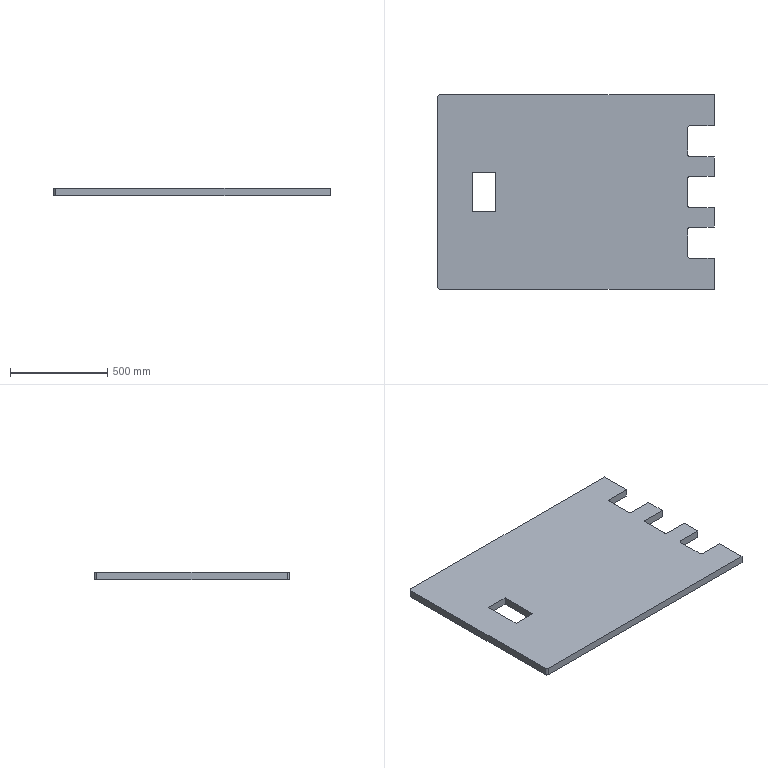Part | SolidWorks | features Extrusion 1, Fillet 1 | 1 solid | 30 faces | box 1420 x 1000 x 40 mm | volume 53251434 mm3 | plane 22 | cylinder 8 | commonest cylinder face diameters 20 x8
STEP:
#1=CARTESIAN_POINT('',(0.,990.,40.));
#2=VERTEX_POINT('',#1);
#3=CARTESIAN_POINT('',(0.,10.,40.));
#4=VERTEX_POINT('',#3);
#5=CARTESIAN_POINT('',(0.,0.,40.));
#6=DIRECTION('',(0.,-1.,0.));
#7=VECTOR('',#6,1000.);
#8=LINE('',#5,#7);
#9=EDGE_CURVE('',#2,#4,#8,.T.);
#10=ORIENTED_EDGE('',*,*,#9,.T.);
#11=CARTESIAN_POINT('',(10.,0.,40.));
#12=VERTEX_POINT('',#11);
#13=CARTESIAN_POINT('',(10.,10.,40.));
#14=DIRECTION('',(0.,0.,1.));
#15=DIRECTION('',(1.,0.,0.));
#16=AXIS2_PLACEMENT_3D('',#13,#14,#15);
#17=CIRCLE('',#16,10.);
#18=EDGE_CURVE('',#4,#12,#17,.T.);
#19=ORIENTED_EDGE('',*,*,#18,.T.);
#20=CARTESIAN_POINT('',(1420.,0.,40.));
#21=VERTEX_POINT('',#20);
#22=CARTESIAN_POINT('',(0.,0.,40.));
#23=DIRECTION('',(1.,0.,0.));
#24=VECTOR('',#23,1000.);
#25=LINE('',#22,#24);
#26=EDGE_CURVE('',#12,#21,#25,.T.);
#27=ORIENTED_EDGE('',*,*,#26,.T.);
#28=CARTESIAN_POINT('',(1420.,160.,40.));
#29=VERTEX_POINT('',#28);
#30=CARTESIAN_POINT('',(1420.,0.,40.));
#31=DIRECTION('',(0.,1.,0.));
#32=VECTOR('',#31,1000.);
#33=LINE('',#30,#32);
#34=EDGE_CURVE('',#21,#29,#33,.T.);
#35=ORIENTED_EDGE('',*,*,#34,.T.);
#36=CARTESIAN_POINT('',(1295.,160.,40.));
#37=VERTEX_POINT('',#36);
#38=CARTESIAN_POINT('',(1295.,160.,40.));
#39=DIRECTION('',(-1.,0.,0.));
#40=VECTOR('',#39,1000.);
#41=LINE('',#38,#40);
#42=EDGE_CURVE('',#29,#37,#41,.T.);
#43=ORIENTED_EDGE('',*,*,#42,.T.);
#44=CARTESIAN_POINT('',(1285.,170.,40.));
#45=VERTEX_POINT('',#44);
#46=CARTESIAN_POINT('',(1295.,170.,40.));
#47=DIRECTION('',(0.,0.,-1.));
#48=DIRECTION('',(1.,0.,0.));
#49=AXIS2_PLACEMENT_3D('',#46,#47,#48);
#50=CIRCLE('',#49,10.);
#51=EDGE_CURVE('',#37,#45,#50,.T.);
#52=ORIENTED_EDGE('',*,*,#51,.T.);
#53=CARTESIAN_POINT('',(1285.,310.,40.));
#54=VERTEX_POINT('',#53);
#55=CARTESIAN_POINT('',(1285.,310.,40.));
#56=DIRECTION('',(0.,1.,0.));
#57=VECTOR('',#56,1000.);
#58=LINE('',#55,#57);
#59=EDGE_CURVE('',#45,#54,#58,.T.);
#60=ORIENTED_EDGE('',*,*,#59,.T.);
#61=CARTESIAN_POINT('',(1295.,320.,40.));
#62=VERTEX_POINT('',#61);
#63=CARTESIAN_POINT('',(1295.,310.,40.));
#64=DIRECTION('',(0.,0.,-1.));
#65=DIRECTION('',(1.,0.,0.));
#66=AXIS2_PLACEMENT_3D('',#63,#64,#65);
#67=CIRCLE('',#66,10.);
#68=EDGE_CURVE('',#54,#62,#67,.T.);
#69=ORIENTED_EDGE('',*,*,#68,.T.);
#70=CARTESIAN_POINT('',(1420.,320.,40.));
#71=VERTEX_POINT('',#70);
#72=CARTESIAN_POINT('',(1420.,320.,40.));
#73=DIRECTION('',(1.,0.,0.));
#74=VECTOR('',#73,1000.);
#75=LINE('',#72,#74);
#76=EDGE_CURVE('',#62,#71,#75,.T.);
#77=ORIENTED_EDGE('',*,*,#76,.T.);
#78=CARTESIAN_POINT('',(1420.,420.,40.));
#79=VERTEX_POINT('',#78);
#80=CARTESIAN_POINT('',(1420.,320.,40.));
#81=DIRECTION('',(0.,1.,0.));
#82=VECTOR('',#81,1000.);
#83=LINE('',#80,#82);
#84=EDGE_CURVE('',#71,#79,#83,.T.);
#85=ORIENTED_EDGE('',*,*,#84,.T.);
#86=CARTESIAN_POINT('',(1295.,420.,40.));
#87=VERTEX_POINT('',#86);
#88=CARTESIAN_POINT('',(1295.,420.,40.));
#89=DIRECTION('',(-1.,0.,0.));
#90=VECTOR('',#89,1000.);
#91=LINE('',#88,#90);
#92=EDGE_CURVE('',#79,#87,#91,.T.);
#93=ORIENTED_EDGE('',*,*,#92,.T.);
#94=CARTESIAN_POINT('',(1285.,430.,40.));
#95=VERTEX_POINT('',#94);
#96=CARTESIAN_POINT('',(1295.,430.,40.));
#97=DIRECTION('',(0.,0.,-1.));
#98=DIRECTION('',(1.,0.,0.));
#99=AXIS2_PLACEMENT_3D('',#96,#97,#98);
#100=CIRCLE('',#99,10.);
#101=EDGE_CURVE('',#87,#95,#100,.T.);
#102=ORIENTED_EDGE('',*,*,#101,.T.);
#103=CARTESIAN_POINT('',(1285.,570.,40.));
#104=VERTEX_POINT('',#103);
#105=CARTESIAN_POINT('',(1285.,570.,40.));
#106=DIRECTION('',(0.,1.,0.));
#107=VECTOR('',#106,1000.);
#108=LINE('',#105,#107);
#109=EDGE_CURVE('',#95,#104,#108,.T.);
#110=ORIENTED_EDGE('',*,*,#109,.T.);
#111=CARTESIAN_POINT('',(1295.,580.,40.));
#112=VERTEX_POINT('',#111);
#113=CARTESIAN_POINT('',(1295.,570.,40.));
#114=DIRECTION('',(0.,0.,-1.));
#115=DIRECTION('',(1.,0.,0.));
#116=AXIS2_PLACEMENT_3D('',#113,#114,#115);
#117=CIRCLE('',#116,10.);
#118=EDGE_CURVE('',#104,#112,#117,.T.);
#119=ORIENTED_EDGE('',*,*,#118,.T.);
#120=CARTESIAN_POINT('',(1420.,580.,40.));
#121=VERTEX_POINT('',#120);
#122=CARTESIAN_POINT('',(1420.,580.,40.));
#123=DIRECTION('',(1.,0.,0.));
#124=VECTOR('',#123,1000.);
#125=LINE('',#122,#124);
#126=EDGE_CURVE('',#112,#121,#125,.T.);
#127=ORIENTED_EDGE('',*,*,#126,.T.);
#128=CARTESIAN_POINT('',(1420.,680.,40.));
#129=VERTEX_POINT('',#128);
#130=CARTESIAN_POINT('',(1420.,580.,40.));
#131=DIRECTION('',(0.,1.,0.));
#132=VECTOR('',#131,1000.);
#133=LINE('',#130,#132);
#134=EDGE_CURVE('',#121,#129,#133,.T.);
#135=ORIENTED_EDGE('',*,*,#134,.T.);
#136=CARTESIAN_POINT('',(1295.,680.,40.));
#137=VERTEX_POINT('',#136);
#138=CARTESIAN_POINT('',(1295.,680.,40.));
#139=DIRECTION('',(-1.,0.,0.));
#140=VECTOR('',#139,1000.);
#141=LINE('',#138,#140);
#142=EDGE_CURVE('',#129,#137,#141,.T.);
#143=ORIENTED_EDGE('',*,*,#142,.T.);
#144=CARTESIAN_POINT('',(1285.,690.,40.));
#145=VERTEX_POINT('',#144);
#146=CARTESIAN_POINT('',(1295.,690.,40.));
#147=DIRECTION('',(0.,0.,-1.));
#148=DIRECTION('',(1.,0.,0.));
#149=AXIS2_PLACEMENT_3D('',#146,#147,#148);
#150=CIRCLE('',#149,10.);
#151=EDGE_CURVE('',#137,#145,#150,.T.);
#152=ORIENTED_EDGE('',*,*,#151,.T.);
#153=CARTESIAN_POINT('',(1285.,830.,40.));
#154=VERTEX_POINT('',#153);
#155=CARTESIAN_POINT('',(1285.,830.,40.));
#156=DIRECTION('',(0.,1.,0.));
#157=VECTOR('',#156,1000.);
#158=LINE('',#155,#157);
#159=EDGE_CURVE('',#145,#154,#158,.T.);
#160=ORIENTED_EDGE('',*,*,#159,.T.);
#161=CARTESIAN_POINT('',(1295.,840.,40.));
#162=VERTEX_POINT('',#161);
#163=CARTESIAN_POINT('',(1295.,830.,40.));
#164=DIRECTION('',(0.,0.,-1.));
#165=DIRECTION('',(1.,0.,0.));
#166=AXIS2_PLACEMENT_3D('',#163,#164,#165);
#167=CIRCLE('',#166,10.);
#168=EDGE_CURVE('',#154,#162,#167,.T.);
#169=ORIENTED_EDGE('',*,*,#168,.T.);
#170=CARTESIAN_POINT('',(1420.,840.,40.));
#171=VERTEX_POINT('',#170);
#172=CARTESIAN_POINT('',(1420.,840.,40.));
#173=DIRECTION('',(1.,0.,0.));
#174=VECTOR('',#173,1000.);
#175=LINE('',#172,#174);
#176=EDGE_CURVE('',#162,#171,#175,.T.);
#177=ORIENTED_EDGE('',*,*,#176,.T.);
#178=CARTESIAN_POINT('',(1420.,1000.,40.));
#179=VERTEX_POINT('',#178);
#180=CARTESIAN_POINT('',(1420.,840.,40.));
#181=DIRECTION('',(0.,1.,0.));
#182=VECTOR('',#181,1000.);
#183=LINE('',#180,#182);
#184=EDGE_CURVE('',#171,#179,#183,.T.);
#185=ORIENTED_EDGE('',*,*,#184,.T.);
#186=CARTESIAN_POINT('',(10.,1000.,40.));
#187=VERTEX_POINT('',#186);
#188=CARTESIAN_POINT('',(0.,1000.,40.));
#189=DIRECTION('',(-1.,0.,0.));
#190=VECTOR('',#189,1000.);
#191=LINE('',#188,#190);
#192=EDGE_CURVE('',#179,#187,#191,.T.);
#193=ORIENTED_EDGE('',*,*,#192,.T.);
#194=CARTESIAN_POINT('',(10.,990.,40.));
#195=DIRECTION('',(0.,0.,1.));
#196=DIRECTION('',(1.,0.,0.));
#197=AXIS2_PLACEMENT_3D('',#194,#195,#196);
#198=CIRCLE('',#197,10.);
#199=EDGE_CURVE('',#187,#2,#198,.T.);
#200=ORIENTED_EDGE('',*,*,#199,.T.);
#201=EDGE_LOOP('',(#10,#19,#27,#35,#43,#52,#60,#69,#77,#85,#93,#102,#110,#119,#127,#135,#143,#152,#160,#169,#177,#185,#193,#200));
#202=FACE_OUTER_BOUND('',#201,.T.);
#203=CARTESIAN_POINT('',(177.,400.,40.));
#204=VERTEX_POINT('',#203);
#205=CARTESIAN_POINT('',(297.,400.,40.));
#206=VERTEX_POINT('',#205);
#207=CARTESIAN_POINT('',(177.,400.,40.));
#208=DIRECTION('',(1.,0.,0.));
#209=VECTOR('',#208,1000.);
#210=LINE('',#207,#209);
#211=EDGE_CURVE('',#204,#206,#210,.T.);
#212=ORIENTED_EDGE('',*,*,#211,.F.);
#213=CARTESIAN_POINT('',(177.,600.,40.));
#214=VERTEX_POINT('',#213);
#215=CARTESIAN_POINT('',(177.,600.,40.));
#216=DIRECTION('',(0.,-1.,0.));
#217=VECTOR('',#216,1000.);
#218=LINE('',#215,#217);
#219=EDGE_CURVE('',#214,#204,#218,.T.);
#220=ORIENTED_EDGE('',*,*,#219,.F.);
#221=CARTESIAN_POINT('',(297.,600.,40.));
#222=VERTEX_POINT('',#221);
#223=CARTESIAN_POINT('',(177.,600.,40.));
#224=DIRECTION('',(-1.,0.,0.));
#225=VECTOR('',#224,1000.);
#226=LINE('',#223,#225);
#227=EDGE_CURVE('',#222,#214,#226,.T.);
#228=ORIENTED_EDGE('',*,*,#227,.F.);
#229=CARTESIAN_POINT('',(297.,600.,40.));
#230=DIRECTION('',(0.,1.,0.));
#231=VECTOR('',#230,1000.);
#232=LINE('',#229,#231);
#233=EDGE_CURVE('',#206,#222,#232,.T.);
#234=ORIENTED_EDGE('',*,*,#233,.F.);
#235=EDGE_LOOP('',(#212,#220,#228,#234));
#236=FACE_BOUND('',#235,.T.);
#237=CARTESIAN_POINT('',(1295.,830.,40.));
#238=DIRECTION('',(0.,0.,1.));
#239=DIRECTION('',(1.,0.,0.));
#240=AXIS2_PLACEMENT_3D('',#237,#238,#239);
#241=PLANE('',#240);
#242=ADVANCED_FACE('',(#202,#236),#241,.T.);
#243=CARTESIAN_POINT('',(10.,0.,0.));
#244=VERTEX_POINT('',#243);
#245=CARTESIAN_POINT('',(1420.,0.,0.));
#246=VERTEX_POINT('',#245);
#247=CARTESIAN_POINT('',(0.,0.,0.));
#248=DIRECTION('',(1.,0.,0.));
#249=VECTOR('',#248,1000.);
#250=LINE('',#247,#249);
#251=EDGE_CURVE('',#244,#246,#250,.T.);
#252=ORIENTED_EDGE('',*,*,#251,.F.);
#253=CARTESIAN_POINT('',(0.,10.,0.));
#254=VERTEX_POINT('',#253);
#255=CARTESIAN_POINT('',(10.,10.,0.));
#256=DIRECTION('',(0.,0.,-1.));
#257=DIRECTION('',(1.,0.,0.));
#258=AXIS2_PLACEMENT_3D('',#255,#256,#257);
#259=CIRCLE('',#258,10.);
#260=EDGE_CURVE('',#244,#254,#259,.T.);
#261=ORIENTED_EDGE('',*,*,#260,.T.);
#262=CARTESIAN_POINT('',(0.,990.,0.));
#263=VERTEX_POINT('',#262);
#264=CARTESIAN_POINT('',(0.,0.,0.));
#265=DIRECTION('',(0.,-1.,0.));
#266=VECTOR('',#265,1000.);
#267=LINE('',#264,#266);
#268=EDGE_CURVE('',#263,#254,#267,.T.);
#269=ORIENTED_EDGE('',*,*,#268,.F.);
#270=CARTESIAN_POINT('',(10.,1000.,0.));
#271=VERTEX_POINT('',#270);
#272=CARTESIAN_POINT('',(10.,990.,0.));
#273=DIRECTION('',(0.,0.,-1.));
#274=DIRECTION('',(1.,0.,0.));
#275=AXIS2_PLACEMENT_3D('',#272,#273,#274);
#276=CIRCLE('',#275,10.);
#277=EDGE_CURVE('',#263,#271,#276,.T.);
#278=ORIENTED_EDGE('',*,*,#277,.T.);
#279=CARTESIAN_POINT('',(1420.,1000.,0.));
#280=VERTEX_POINT('',#279);
#281=CARTESIAN_POINT('',(0.,1000.,0.));
#282=DIRECTION('',(-1.,0.,0.));
#283=VECTOR('',#282,1000.);
#284=LINE('',#281,#283);
#285=EDGE_CURVE('',#280,#271,#284,.T.);
#286=ORIENTED_EDGE('',*,*,#285,.F.);
#287=CARTESIAN_POINT('',(1420.,840.,0.));
#288=VERTEX_POINT('',#287);
#289=CARTESIAN_POINT('',(1420.,840.,0.));
#290=DIRECTION('',(0.,1.,0.));
#291=VECTOR('',#290,1000.);
#292=LINE('',#289,#291);
#293=EDGE_CURVE('',#288,#280,#292,.T.);
#294=ORIENTED_EDGE('',*,*,#293,.F.);
#295=CARTESIAN_POINT('',(1295.,840.,0.));
#296=VERTEX_POINT('',#295);
#297=CARTESIAN_POINT('',(1420.,840.,0.));
#298=DIRECTION('',(1.,0.,0.));
#299=VECTOR('',#298,1000.);
#300=LINE('',#297,#299);
#301=EDGE_CURVE('',#296,#288,#300,.T.);
#302=ORIENTED_EDGE('',*,*,#301,.F.);
#303=CARTESIAN_POINT('',(1285.,830.,0.));
#304=VERTEX_POINT('',#303);
#305=CARTESIAN_POINT('',(1295.,830.,0.));
#306=DIRECTION('',(0.,0.,-1.));
#307=DIRECTION('',(1.,0.,0.));
#308=AXIS2_PLACEMENT_3D('',#305,#306,#307);
#309=CIRCLE('',#308,10.);
#310=EDGE_CURVE('',#304,#296,#309,.T.);
#311=ORIENTED_EDGE('',*,*,#310,.F.);
#312=CARTESIAN_POINT('',(1285.,690.,0.));
#313=VERTEX_POINT('',#312);
#314=CARTESIAN_POINT('',(1285.,830.,0.));
#315=DIRECTION('',(0.,1.,0.));
#316=VECTOR('',#315,1000.);
#317=LINE('',#314,#316);
#318=EDGE_CURVE('',#313,#304,#317,.T.);
#319=ORIENTED_EDGE('',*,*,#318,.F.);
#320=CARTESIAN_POINT('',(1295.,680.,0.));
#321=VERTEX_POINT('',#320);
#322=CARTESIAN_POINT('',(1295.,690.,0.));
#323=DIRECTION('',(0.,0.,-1.));
#324=DIRECTION('',(1.,0.,0.));
#325=AXIS2_PLACEMENT_3D('',#322,#323,#324);
#326=CIRCLE('',#325,10.);
#327=EDGE_CURVE('',#321,#313,#326,.T.);
#328=ORIENTED_EDGE('',*,*,#327,.F.);
#329=CARTESIAN_POINT('',(1420.,680.,0.));
#330=VERTEX_POINT('',#329);
#331=CARTESIAN_POINT('',(1295.,680.,0.));
#332=DIRECTION('',(-1.,0.,0.));
#333=VECTOR('',#332,1000.);
#334=LINE('',#331,#333);
#335=EDGE_CURVE('',#330,#321,#334,.T.);
#336=ORIENTED_EDGE('',*,*,#335,.F.);
#337=CARTESIAN_POINT('',(1420.,580.,0.));
#338=VERTEX_POINT('',#337);
#339=CARTESIAN_POINT('',(1420.,580.,0.));
#340=DIRECTION('',(0.,1.,0.));
#341=VECTOR('',#340,1000.);
#342=LINE('',#339,#341);
#343=EDGE_CURVE('',#338,#330,#342,.T.);
#344=ORIENTED_EDGE('',*,*,#343,.F.);
#345=CARTESIAN_POINT('',(1295.,580.,0.));
#346=VERTEX_POINT('',#345);
#347=CARTESIAN_POINT('',(1420.,580.,0.));
#348=DIRECTION('',(1.,0.,0.));
#349=VECTOR('',#348,1000.);
#350=LINE('',#347,#349);
#351=EDGE_CURVE('',#346,#338,#350,.T.);
#352=ORIENTED_EDGE('',*,*,#351,.F.);
#353=CARTESIAN_POINT('',(1285.,570.,0.));
#354=VERTEX_POINT('',#353);
#355=CARTESIAN_POINT('',(1295.,570.,0.));
#356=DIRECTION('',(0.,0.,-1.));
#357=DIRECTION('',(1.,0.,0.));
#358=AXIS2_PLACEMENT_3D('',#355,#356,#357);
#359=CIRCLE('',#358,10.);
#360=EDGE_CURVE('',#354,#346,#359,.T.);
#361=ORIENTED_EDGE('',*,*,#360,.F.);
#362=CARTESIAN_POINT('',(1285.,430.,0.));
#363=VERTEX_POINT('',#362);
#364=CARTESIAN_POINT('',(1285.,570.,0.));
#365=DIRECTION('',(0.,1.,0.));
#366=VECTOR('',#365,1000.);
#367=LINE('',#364,#366);
#368=EDGE_CURVE('',#363,#354,#367,.T.);
#369=ORIENTED_EDGE('',*,*,#368,.F.);
#370=CARTESIAN_POINT('',(1295.,420.,0.));
#371=VERTEX_POINT('',#370);
#372=CARTESIAN_POINT('',(1295.,430.,0.));
#373=DIRECTION('',(0.,0.,-1.));
#374=DIRECTION('',(1.,0.,0.));
#375=AXIS2_PLACEMENT_3D('',#372,#373,#374);
#376=CIRCLE('',#375,10.);
#377=EDGE_CURVE('',#371,#363,#376,.T.);
#378=ORIENTED_EDGE('',*,*,#377,.F.);
#379=CARTESIAN_POINT('',(1420.,420.,0.));
#380=VERTEX_POINT('',#379);
#381=CARTESIAN_POINT('',(1295.,420.,0.));
#382=DIRECTION('',(-1.,0.,0.));
#383=VECTOR('',#382,1000.);
#384=LINE('',#381,#383);
#385=EDGE_CURVE('',#380,#371,#384,.T.);
#386=ORIENTED_EDGE('',*,*,#385,.F.);
#387=CARTESIAN_POINT('',(1420.,320.,0.));
#388=VERTEX_POINT('',#387);
#389=CARTESIAN_POINT('',(1420.,320.,0.));
#390=DIRECTION('',(0.,1.,0.));
#391=VECTOR('',#390,1000.);
#392=LINE('',#389,#391);
#393=EDGE_CURVE('',#388,#380,#392,.T.);
#394=ORIENTED_EDGE('',*,*,#393,.F.);
#395=CARTESIAN_POINT('',(1295.,320.,0.));
#396=VERTEX_POINT('',#395);
#397=CARTESIAN_POINT('',(1420.,320.,0.));
#398=DIRECTION('',(1.,0.,0.));
#399=VECTOR('',#398,1000.);
#400=LINE('',#397,#399);
#401=EDGE_CURVE('',#396,#388,#400,.T.);
#402=ORIENTED_EDGE('',*,*,#401,.F.);
#403=CARTESIAN_POINT('',(1285.,310.,0.));
#404=VERTEX_POINT('',#403);
#405=CARTESIAN_POINT('',(1295.,310.,0.));
#406=DIRECTION('',(0.,0.,-1.));
#407=DIRECTION('',(1.,0.,0.));
#408=AXIS2_PLACEMENT_3D('',#405,#406,#407);
#409=CIRCLE('',#408,10.);
#410=EDGE_CURVE('',#404,#396,#409,.T.);
#411=ORIENTED_EDGE('',*,*,#410,.F.);
#412=CARTESIAN_POINT('',(1285.,170.,0.));
#413=VERTEX_POINT('',#412);
#414=CARTESIAN_POINT('',(1285.,310.,0.));
#415=DIRECTION('',(0.,1.,0.));
#416=VECTOR('',#415,1000.);
#417=LINE('',#414,#416);
#418=EDGE_CURVE('',#413,#404,#417,.T.);
#419=ORIENTED_EDGE('',*,*,#418,.F.);
#420=CARTESIAN_POINT('',(1295.,160.,0.));
#421=VERTEX_POINT('',#420);
#422=CARTESIAN_POINT('',(1295.,170.,0.));
#423=DIRECTION('',(0.,0.,-1.));
#424=DIRECTION('',(1.,0.,0.));
#425=AXIS2_PLACEMENT_3D('',#422,#423,#424);
#426=CIRCLE('',#425,10.);
#427=EDGE_CURVE('',#421,#413,#426,.T.);
#428=ORIENTED_EDGE('',*,*,#427,.F.);
#429=CARTESIAN_POINT('',(1420.,160.,0.));
#430=VERTEX_POINT('',#429);
#431=CARTESIAN_POINT('',(1295.,160.,0.));
#432=DIRECTION('',(-1.,0.,0.));
#433=VECTOR('',#432,1000.);
#434=LINE('',#431,#433);
#435=EDGE_CURVE('',#430,#421,#434,.T.);
#436=ORIENTED_EDGE('',*,*,#435,.F.);
#437=CARTESIAN_POINT('',(1420.,0.,0.));
#438=DIRECTION('',(0.,1.,0.));
#439=VECTOR('',#438,1000.);
#440=LINE('',#437,#439);
#441=EDGE_CURVE('',#246,#430,#440,.T.);
#442=ORIENTED_EDGE('',*,*,#441,.F.);
#443=EDGE_LOOP('',(#252,#261,#269,#278,#286,#294,#302,#311,#319,#328,#336,#344,#352,#361,#369,#378,#386,#394,#402,#411,#419,#428,#436,#442));
#444=FACE_OUTER_BOUND('',#443,.T.);
#445=CARTESIAN_POINT('',(177.,600.,0.));
#446=VERTEX_POINT('',#445);
#447=CARTESIAN_POINT('',(177.,400.,0.));
#448=VERTEX_POINT('',#447);
#449=CARTESIAN_POINT('',(177.,600.,0.));
#450=DIRECTION('',(0.,-1.,0.));
#451=VECTOR('',#450,1000.);
#452=LINE('',#449,#451);
#453=EDGE_CURVE('',#446,#448,#452,.T.);
#454=ORIENTED_EDGE('',*,*,#453,.T.);
#455=CARTESIAN_POINT('',(297.,400.,0.));
#456=VERTEX_POINT('',#455);
#457=CARTESIAN_POINT('',(177.,400.,0.));
#458=DIRECTION('',(1.,0.,0.));
#459=VECTOR('',#458,1000.);
#460=LINE('',#457,#459);
#461=EDGE_CURVE('',#448,#456,#460,.T.);
#462=ORIENTED_EDGE('',*,*,#461,.T.);
#463=CARTESIAN_POINT('',(297.,600.,0.));
#464=VERTEX_POINT('',#463);
#465=CARTESIAN_POINT('',(297.,600.,0.));
#466=DIRECTION('',(0.,1.,0.));
#467=VECTOR('',#466,1000.);
#468=LINE('',#465,#467);
#469=EDGE_CURVE('',#456,#464,#468,.T.);
#470=ORIENTED_EDGE('',*,*,#469,.T.);
#471=CARTESIAN_POINT('',(177.,600.,0.));
#472=DIRECTION('',(-1.,0.,0.));
#473=VECTOR('',#472,1000.);
#474=LINE('',#471,#473);
#475=EDGE_CURVE('',#464,#446,#474,.T.);
#476=ORIENTED_EDGE('',*,*,#475,.T.);
#477=EDGE_LOOP('',(#454,#462,#470,#476));
#478=FACE_BOUND('',#477,.T.);
#479=CARTESIAN_POINT('',(1295.,830.,0.));
#480=DIRECTION('',(0.,0.,1.));
#481=DIRECTION('',(1.,0.,0.));
#482=AXIS2_PLACEMENT_3D('',#479,#480,#481);
#483=PLANE('',#482);
#484=ADVANCED_FACE('',(#444,#478),#483,.F.);
#485=ORIENTED_EDGE('',*,*,#268,.T.);
#486=CARTESIAN_POINT('',(0.,10.,40.));
#487=DIRECTION('',(0.,0.,1.));
#488=VECTOR('',#487,1000.);
#489=LINE('',#486,#488);
#490=EDGE_CURVE('',#254,#4,#489,.T.);
#491=ORIENTED_EDGE('',*,*,#490,.T.);
#492=ORIENTED_EDGE('',*,*,#9,.F.);
#493=CARTESIAN_POINT('',(0.,990.,40.));
#494=DIRECTION('',(0.,0.,-1.));
#495=VECTOR('',#494,1000.);
#496=LINE('',#493,#495);
#497=EDGE_CURVE('',#2,#263,#496,.T.);
#498=ORIENTED_EDGE('',*,*,#497,.T.);
#499=EDGE_LOOP('',(#485,#491,#492,#498));
#500=FACE_OUTER_BOUND('',#499,.T.);
#501=CARTESIAN_POINT('',(0.,0.,40.));
#502=DIRECTION('',(1.,0.,0.));
#503=DIRECTION('',(0.,0.,-1.));
#504=AXIS2_PLACEMENT_3D('',#501,#502,#503);
#505=PLANE('',#504);
#506=ADVANCED_FACE('',(#500),#505,.F.);
#507=ORIENTED_EDGE('',*,*,#26,.F.);
#508=CARTESIAN_POINT('',(10.,0.,40.));
#509=DIRECTION('',(0.,0.,-1.));
#510=VECTOR('',#509,1000.);
#511=LINE('',#508,#510);
#512=EDGE_CURVE('',#12,#244,#511,.T.);
#513=ORIENTED_EDGE('',*,*,#512,.T.);
#514=ORIENTED_EDGE('',*,*,#251,.T.);
#515=CARTESIAN_POINT('',(1420.,0.,40.));
#516=DIRECTION('',(0.,0.,-1.));
#517=VECTOR('',#516,1000.);
#518=LINE('',#515,#517);
#519=EDGE_CURVE('',#21,#246,#518,.T.);
#520=ORIENTED_EDGE('',*,*,#519,.F.);
#521=EDGE_LOOP('',(#507,#513,#514,#520));
#522=FACE_OUTER_BOUND('',#521,.T.);
#523=CARTESIAN_POINT('',(0.,0.,40.));
#524=DIRECTION('',(0.,1.,0.));
#525=DIRECTION('',(0.,0.,1.));
#526=AXIS2_PLACEMENT_3D('',#523,#524,#525);
#527=PLANE('',#526);
#528=ADVANCED_FACE('',(#522),#527,.F.);
#529=ORIENTED_EDGE('',*,*,#441,.T.);
#530=CARTESIAN_POINT('',(1420.,160.,40.));
#531=DIRECTION('',(0.,0.,-1.));
#532=VECTOR('',#531,1000.);
#533=LINE('',#530,#532);
#534=EDGE_CURVE('',#29,#430,#533,.T.);
#535=ORIENTED_EDGE('',*,*,#534,.F.);
#536=ORIENTED_EDGE('',*,*,#34,.F.);
#537=ORIENTED_EDGE('',*,*,#519,.T.);
#538=EDGE_LOOP('',(#529,#535,#536,#537));
#539=FACE_OUTER_BOUND('',#538,.T.);
#540=CARTESIAN_POINT('',(1420.,0.,40.));
#541=DIRECTION('',(-1.,0.,0.));
#542=DIRECTION('',(0.,0.,1.));
#543=AXIS2_PLACEMENT_3D('',#540,#541,#542);
#544=PLANE('',#543);
#545=ADVANCED_FACE('',(#539),#544,.F.);
#546=ORIENTED_EDGE('',*,*,#435,.T.);
#547=CARTESIAN_POINT('',(1295.,160.,40.));
#548=DIRECTION('',(0.,0.,-1.));
#549=VECTOR('',#548,1000.);
#550=LINE('',#547,#549);
#551=EDGE_CURVE('',#37,#421,#550,.T.);
#552=ORIENTED_EDGE('',*,*,#551,.F.);
#553=ORIENTED_EDGE('',*,*,#42,.F.);
#554=ORIENTED_EDGE('',*,*,#534,.T.);
#555=EDGE_LOOP('',(#546,#552,#553,#554));
#556=FACE_OUTER_BOUND('',#555,.T.);
#557=CARTESIAN_POINT('',(1295.,160.,40.));
#558=DIRECTION('',(0.,-1.,0.));
#559=DIRECTION('',(0.,0.,-1.));
#560=AXIS2_PLACEMENT_3D('',#557,#558,#559);
#561=PLANE('',#560);
#562=ADVANCED_FACE('',(#556),#561,.F.);
#563=ORIENTED_EDGE('',*,*,#427,.T.);
#564=CARTESIAN_POINT('',(1285.,170.,40.));
#565=DIRECTION('',(0.,0.,-1.));
#566=VECTOR('',#565,1000.);
#567=LINE('',#564,#566);
#568=EDGE_CURVE('',#45,#413,#567,.T.);
#569=ORIENTED_EDGE('',*,*,#568,.F.);
#570=ORIENTED_EDGE('',*,*,#51,.F.);
#571=ORIENTED_EDGE('',*,*,#551,.T.);
#572=EDGE_LOOP('',(#563,#569,#570,#571));
#573=FACE_OUTER_BOUND('',#572,.T.);
#574=CARTESIAN_POINT('',(1295.,170.,40.));
#575=DIRECTION('',(0.,0.,-1.));
#576=DIRECTION('',(-1.,0.,0.));
#577=AXIS2_PLACEMENT_3D('',#574,#575,#576);
#578=CYLINDRICAL_SURFACE('',#577,10.);
#579=ADVANCED_FACE('',(#573),#578,.F.);
#580=ORIENTED_EDGE('',*,*,#418,.T.);
#581=CARTESIAN_POINT('',(1285.,310.,40.));
#582=DIRECTION('',(0.,0.,-1.));
#583=VECTOR('',#582,1000.);
#584=LINE('',#581,#583);
#585=EDGE_CURVE('',#54,#404,#584,.T.);
#586=ORIENTED_EDGE('',*,*,#585,.F.);
#587=ORIENTED_EDGE('',*,*,#59,.F.);
#588=ORIENTED_EDGE('',*,*,#568,.T.);
#589=EDGE_LOOP('',(#580,#586,#587,#588));
#590=FACE_OUTER_BOUND('',#589,.T.);
#591=CARTESIAN_POINT('',(1285.,310.,40.));
#592=DIRECTION('',(-1.,0.,0.));
#593=DIRECTION('',(0.,0.,1.));
#594=AXIS2_PLACEMENT_3D('',#591,#592,#593);
#595=PLANE('',#594);
#596=ADVANCED_FACE('',(#590),#595,.F.);
#597=ORIENTED_EDGE('',*,*,#410,.T.);
#598=CARTESIAN_POINT('',(1295.,320.,40.));
#599=DIRECTION('',(0.,0.,-1.));
#600=VECTOR('',#599,1000.);
#601=LINE('',#598,#600);
#602=EDGE_CURVE('',#62,#396,#601,.T.);
#603=ORIENTED_EDGE('',*,*,#602,.F.);
#604=ORIENTED_EDGE('',*,*,#68,.F.);
#605=ORIENTED_EDGE('',*,*,#585,.T.);
#606=EDGE_LOOP('',(#597,#603,#604,#605));
#607=FACE_OUTER_BOUND('',#606,.T.);
#608=CARTESIAN_POINT('',(1295.,310.,40.));
#609=DIRECTION('',(0.,0.,-1.));
#610=DIRECTION('',(-1.,0.,0.));
#611=AXIS2_PLACEMENT_3D('',#608,#609,#610);
#612=CYLINDRICAL_SURFACE('',#611,10.);
#613=ADVANCED_FACE('',(#607),#612,.F.);
#614=ORIENTED_EDGE('',*,*,#401,.T.);
#615=CARTESIAN_POINT('',(1420.,320.,40.));
#616=DIRECTION('',(0.,0.,-1.));
#617=VECTOR('',#616,1000.);
#618=LINE('',#615,#617);
#619=EDGE_CURVE('',#71,#388,#618,.T.);
#620=ORIENTED_EDGE('',*,*,#619,.F.);
#621=ORIENTED_EDGE('',*,*,#76,.F.);
#622=ORIENTED_EDGE('',*,*,#602,.T.);
#623=EDGE_LOOP('',(#614,#620,#621,#622));
#624=FACE_OUTER_BOUND('',#623,.T.);
#625=CARTESIAN_POINT('',(1420.,320.,40.));
#626=DIRECTION('',(0.,1.,0.));
#627=DIRECTION('',(-1.,0.,0.));
#628=AXIS2_PLACEMENT_3D('',#625,#626,#627);
#629=PLANE('',#628);
#630=ADVANCED_FACE('',(#624),#629,.F.);
#631=ORIENTED_EDGE('',*,*,#393,.T.);
#632=CARTESIAN_POINT('',(1420.,420.,40.));
#633=DIRECTION('',(0.,0.,-1.));
#634=VECTOR('',#633,1000.);
#635=LINE('',#632,#634);
#636=EDGE_CURVE('',#79,#380,#635,.T.);
#637=ORIENTED_EDGE('',*,*,#636,.F.);
#638=ORIENTED_EDGE('',*,*,#84,.F.);
#639=ORIENTED_EDGE('',*,*,#619,.T.);
#640=EDGE_LOOP('',(#631,#637,#638,#639));
#641=FACE_OUTER_BOUND('',#640,.T.);
#642=CARTESIAN_POINT('',(1420.,320.,40.));
#643=DIRECTION('',(-1.,0.,0.));
#644=DIRECTION('',(0.,-1.,0.));
#645=AXIS2_PLACEMENT_3D('',#642,#643,#644);
#646=PLANE('',#645);
#647=ADVANCED_FACE('',(#641),#646,.F.);
#648=ORIENTED_EDGE('',*,*,#385,.T.);
#649=CARTESIAN_POINT('',(1295.,420.,40.));
#650=DIRECTION('',(0.,0.,-1.));
#651=VECTOR('',#650,1000.);
#652=LINE('',#649,#651);
#653=EDGE_CURVE('',#87,#371,#652,.T.);
#654=ORIENTED_EDGE('',*,*,#653,.F.);
#655=ORIENTED_EDGE('',*,*,#92,.F.);
#656=ORIENTED_EDGE('',*,*,#636,.T.);
#657=EDGE_LOOP('',(#648,#654,#655,#656));
#658=FACE_OUTER_BOUND('',#657,.T.);
#659=CARTESIAN_POINT('',(1295.,420.,40.));
#660=DIRECTION('',(0.,-1.,0.));
#661=DIRECTION('',(0.,0.,-1.));
#662=AXIS2_PLACEMENT_3D('',#659,#660,#661);
#663=PLANE('',#662);
#664=ADVANCED_FACE('',(#658),#663,.F.);
#665=ORIENTED_EDGE('',*,*,#377,.T.);
#666=CARTESIAN_POINT('',(1285.,430.,40.));
#667=DIRECTION('',(0.,0.,-1.));
#668=VECTOR('',#667,1000.);
#669=LINE('',#666,#668);
#670=EDGE_CURVE('',#95,#363,#669,.T.);
#671=ORIENTED_EDGE('',*,*,#670,.F.);
#672=ORIENTED_EDGE('',*,*,#101,.F.);
#673=ORIENTED_EDGE('',*,*,#653,.T.);
#674=EDGE_LOOP('',(#665,#671,#672,#673));
#675=FACE_OUTER_BOUND('',#674,.T.);
#676=CARTESIAN_POINT('',(1295.,430.,40.));
#677=DIRECTION('',(0.,0.,-1.));
#678=DIRECTION('',(-1.,0.,0.));
#679=AXIS2_PLACEMENT_3D('',#676,#677,#678);
#680=CYLINDRICAL_SURFACE('',#679,10.);
#681=ADVANCED_FACE('',(#675),#680,.F.);
#682=ORIENTED_EDGE('',*,*,#368,.T.);
#683=CARTESIAN_POINT('',(1285.,570.,40.));
#684=DIRECTION('',(0.,0.,-1.));
#685=VECTOR('',#684,1000.);
#686=LINE('',#683,#685);
#687=EDGE_CURVE('',#104,#354,#686,.T.);
#688=ORIENTED_EDGE('',*,*,#687,.F.);
#689=ORIENTED_EDGE('',*,*,#109,.F.);
#690=ORIENTED_EDGE('',*,*,#670,.T.);
#691=EDGE_LOOP('',(#682,#688,#689,#690));
#692=FACE_OUTER_BOUND('',#691,.T.);
#693=CARTESIAN_POINT('',(1285.,570.,40.));
#694=DIRECTION('',(-1.,0.,0.));
#695=DIRECTION('',(0.,0.,1.));
#696=AXIS2_PLACEMENT_3D('',#693,#694,#695);
#697=PLANE('',#696);
#698=ADVANCED_FACE('',(#692),#697,.F.);
#699=ORIENTED_EDGE('',*,*,#360,.T.);
#700=CARTESIAN_POINT('',(1295.,580.,40.));
#701=DIRECTION('',(0.,0.,-1.));
#702=VECTOR('',#701,1000.);
#703=LINE('',#700,#702);
#704=EDGE_CURVE('',#112,#346,#703,.T.);
#705=ORIENTED_EDGE('',*,*,#704,.F.);
#706=ORIENTED_EDGE('',*,*,#118,.F.);
#707=ORIENTED_EDGE('',*,*,#687,.T.);
#708=EDGE_LOOP('',(#699,#705,#706,#707));
#709=FACE_OUTER_BOUND('',#708,.T.);
#710=CARTESIAN_POINT('',(1295.,570.,40.));
#711=DIRECTION('',(0.,0.,-1.));
#712=DIRECTION('',(-1.,0.,0.));
#713=AXIS2_PLACEMENT_3D('',#710,#711,#712);
#714=CYLINDRICAL_SURFACE('',#713,10.);
#715=ADVANCED_FACE('',(#709),#714,.F.);
#716=ORIENTED_EDGE('',*,*,#351,.T.);
#717=CARTESIAN_POINT('',(1420.,580.,40.));
#718=DIRECTION('',(0.,0.,-1.));
#719=VECTOR('',#718,1000.);
#720=LINE('',#717,#719);
#721=EDGE_CURVE('',#121,#338,#720,.T.);
#722=ORIENTED_EDGE('',*,*,#721,.F.);
#723=ORIENTED_EDGE('',*,*,#126,.F.);
#724=ORIENTED_EDGE('',*,*,#704,.T.);
#725=EDGE_LOOP('',(#716,#722,#723,#724));
#726=FACE_OUTER_BOUND('',#725,.T.);
#727=CARTESIAN_POINT('',(1420.,580.,40.));
#728=DIRECTION('',(0.,1.,0.));
#729=DIRECTION('',(-1.,0.,0.));
#730=AXIS2_PLACEMENT_3D('',#727,#728,#729);
#731=PLANE('',#730);
#732=ADVANCED_FACE('',(#726),#731,.F.);
#733=ORIENTED_EDGE('',*,*,#343,.T.);
#734=CARTESIAN_POINT('',(1420.,680.,40.));
#735=DIRECTION('',(0.,0.,-1.));
#736=VECTOR('',#735,1000.);
#737=LINE('',#734,#736);
#738=EDGE_CURVE('',#129,#330,#737,.T.);
#739=ORIENTED_EDGE('',*,*,#738,.F.);
#740=ORIENTED_EDGE('',*,*,#134,.F.);
#741=ORIENTED_EDGE('',*,*,#721,.T.);
#742=EDGE_LOOP('',(#733,#739,#740,#741));
#743=FACE_OUTER_BOUND('',#742,.T.);
#744=CARTESIAN_POINT('',(1420.,580.,40.));
#745=DIRECTION('',(-1.,0.,0.));
#746=DIRECTION('',(0.,0.,1.));
#747=AXIS2_PLACEMENT_3D('',#744,#745,#746);
#748=PLANE('',#747);
#749=ADVANCED_FACE('',(#743),#748,.F.);
#750=ORIENTED_EDGE('',*,*,#335,.T.);
#751=CARTESIAN_POINT('',(1295.,680.,40.));
#752=DIRECTION('',(0.,0.,-1.));
#753=VECTOR('',#752,1000.);
#754=LINE('',#751,#753);
#755=EDGE_CURVE('',#137,#321,#754,.T.);
#756=ORIENTED_EDGE('',*,*,#755,.F.);
#757=ORIENTED_EDGE('',*,*,#142,.F.);
#758=ORIENTED_EDGE('',*,*,#738,.T.);
#759=EDGE_LOOP('',(#750,#756,#757,#758));
#760=FACE_OUTER_BOUND('',#759,.T.);
#761=CARTESIAN_POINT('',(1295.,680.,40.));
#762=DIRECTION('',(0.,-1.,0.));
#763=DIRECTION('',(0.,0.,-1.));
#764=AXIS2_PLACEMENT_3D('',#761,#762,#763);
#765=PLANE('',#764);
#766=ADVANCED_FACE('',(#760),#765,.F.);
#767=ORIENTED_EDGE('',*,*,#327,.T.);
#768=CARTESIAN_POINT('',(1285.,690.,40.));
#769=DIRECTION('',(0.,0.,-1.));
#770=VECTOR('',#769,1000.);
#771=LINE('',#768,#770);
#772=EDGE_CURVE('',#145,#313,#771,.T.);
#773=ORIENTED_EDGE('',*,*,#772,.F.);
#774=ORIENTED_EDGE('',*,*,#151,.F.);
#775=ORIENTED_EDGE('',*,*,#755,.T.);
#776=EDGE_LOOP('',(#767,#773,#774,#775));
#777=FACE_OUTER_BOUND('',#776,.T.);
#778=CARTESIAN_POINT('',(1295.,690.,40.));
#779=DIRECTION('',(0.,0.,-1.));
#780=DIRECTION('',(-1.,0.,0.));
#781=AXIS2_PLACEMENT_3D('',#778,#779,#780);
#782=CYLINDRICAL_SURFACE('',#781,10.);
#783=ADVANCED_FACE('',(#777),#782,.F.);
#784=ORIENTED_EDGE('',*,*,#318,.T.);
#785=CARTESIAN_POINT('',(1285.,830.,40.));
#786=DIRECTION('',(0.,0.,-1.));
#787=VECTOR('',#786,1000.);
#788=LINE('',#785,#787);
#789=EDGE_CURVE('',#154,#304,#788,.T.);
#790=ORIENTED_EDGE('',*,*,#789,.F.);
#791=ORIENTED_EDGE('',*,*,#159,.F.);
#792=ORIENTED_EDGE('',*,*,#772,.T.);
#793=EDGE_LOOP('',(#784,#790,#791,#792));
#794=FACE_OUTER_BOUND('',#793,.T.);
#795=CARTESIAN_POINT('',(1285.,830.,40.));
#796=DIRECTION('',(-1.,0.,0.));
#797=DIRECTION('',(0.,0.,1.));
#798=AXIS2_PLACEMENT_3D('',#795,#796,#797);
#799=PLANE('',#798);
#800=ADVANCED_FACE('',(#794),#799,.F.);
#801=ORIENTED_EDGE('',*,*,#310,.T.);
#802=CARTESIAN_POINT('',(1295.,840.,40.));
#803=DIRECTION('',(0.,0.,-1.));
#804=VECTOR('',#803,1000.);
#805=LINE('',#802,#804);
#806=EDGE_CURVE('',#162,#296,#805,.T.);
#807=ORIENTED_EDGE('',*,*,#806,.F.);
#808=ORIENTED_EDGE('',*,*,#168,.F.);
#809=ORIENTED_EDGE('',*,*,#789,.T.);
#810=EDGE_LOOP('',(#801,#807,#808,#809));
#811=FACE_OUTER_BOUND('',#810,.T.);
#812=CARTESIAN_POINT('',(1295.,830.,40.));
#813=DIRECTION('',(0.,0.,-1.));
#814=DIRECTION('',(-1.,0.,0.));
#815=AXIS2_PLACEMENT_3D('',#812,#813,#814);
#816=CYLINDRICAL_SURFACE('',#815,10.);
#817=ADVANCED_FACE('',(#811),#816,.F.);
#818=ORIENTED_EDGE('',*,*,#301,.T.);
#819=CARTESIAN_POINT('',(1420.,840.,40.));
#820=DIRECTION('',(0.,0.,-1.));
#821=VECTOR('',#820,1000.);
#822=LINE('',#819,#821);
#823=EDGE_CURVE('',#171,#288,#822,.T.);
#824=ORIENTED_EDGE('',*,*,#823,.F.);
#825=ORIENTED_EDGE('',*,*,#176,.F.);
#826=ORIENTED_EDGE('',*,*,#806,.T.);
#827=EDGE_LOOP('',(#818,#824,#825,#826));
#828=FACE_OUTER_BOUND('',#827,.T.);
#829=CARTESIAN_POINT('',(1420.,840.,40.));
#830=DIRECTION('',(0.,1.,0.));
#831=DIRECTION('',(-1.,0.,0.));
#832=AXIS2_PLACEMENT_3D('',#829,#830,#831);
#833=PLANE('',#832);
#834=ADVANCED_FACE('',(#828),#833,.F.);
#835=ORIENTED_EDGE('',*,*,#293,.T.);
#836=CARTESIAN_POINT('',(1420.,1000.,40.));
#837=DIRECTION('',(0.,0.,-1.));
#838=VECTOR('',#837,1000.);
#839=LINE('',#836,#838);
#840=EDGE_CURVE('',#179,#280,#839,.T.);
#841=ORIENTED_EDGE('',*,*,#840,.F.);
#842=ORIENTED_EDGE('',*,*,#184,.F.);
#843=ORIENTED_EDGE('',*,*,#823,.T.);
#844=EDGE_LOOP('',(#835,#841,#842,#843));
#845=FACE_OUTER_BOUND('',#844,.T.);
#846=CARTESIAN_POINT('',(1420.,840.,40.));
#847=DIRECTION('',(-1.,0.,0.));
#848=DIRECTION('',(0.,0.,1.));
#849=AXIS2_PLACEMENT_3D('',#846,#847,#848);
#850=PLANE('',#849);
#851=ADVANCED_FACE('',(#845),#850,.F.);
#852=ORIENTED_EDGE('',*,*,#285,.T.);
#853=CARTESIAN_POINT('',(10.,1000.,40.));
#854=DIRECTION('',(0.,0.,1.));
#855=VECTOR('',#854,1000.);
#856=LINE('',#853,#855);
#857=EDGE_CURVE('',#271,#187,#856,.T.);
#858=ORIENTED_EDGE('',*,*,#857,.T.);
#859=ORIENTED_EDGE('',*,*,#192,.F.);
#860=ORIENTED_EDGE('',*,*,#840,.T.);
#861=EDGE_LOOP('',(#852,#858,#859,#860));
#862=FACE_OUTER_BOUND('',#861,.T.);
#863=CARTESIAN_POINT('',(0.,1000.,40.));
#864=DIRECTION('',(0.,-1.,0.));
#865=DIRECTION('',(0.,0.,-1.));
#866=AXIS2_PLACEMENT_3D('',#863,#864,#865);
#867=PLANE('',#866);
#868=ADVANCED_FACE('',(#862),#867,.F.);
#869=ORIENTED_EDGE('',*,*,#453,.F.);
#870=CARTESIAN_POINT('',(177.,600.,40.));
#871=DIRECTION('',(0.,0.,-1.));
#872=VECTOR('',#871,1000.);
#873=LINE('',#870,#872);
#874=EDGE_CURVE('',#214,#446,#873,.T.);
#875=ORIENTED_EDGE('',*,*,#874,.F.);
#876=ORIENTED_EDGE('',*,*,#219,.T.);
#877=CARTESIAN_POINT('',(177.,400.,40.));
#878=DIRECTION('',(0.,0.,-1.));
#879=VECTOR('',#878,1000.);
#880=LINE('',#877,#879);
#881=EDGE_CURVE('',#204,#448,#880,.T.);
#882=ORIENTED_EDGE('',*,*,#881,.T.);
#883=EDGE_LOOP('',(#869,#875,#876,#882));
#884=FACE_OUTER_BOUND('',#883,.T.);
#885=CARTESIAN_POINT('',(177.,600.,40.));
#886=DIRECTION('',(1.,0.,0.));
#887=DIRECTION('',(0.,1.,0.));
#888=AXIS2_PLACEMENT_3D('',#885,#886,#887);
#889=PLANE('',#888);
#890=ADVANCED_FACE('',(#884),#889,.T.);
#891=ORIENTED_EDGE('',*,*,#461,.F.);
#892=ORIENTED_EDGE('',*,*,#881,.F.);
#893=ORIENTED_EDGE('',*,*,#211,.T.);
#894=CARTESIAN_POINT('',(297.,400.,40.));
#895=DIRECTION('',(0.,0.,-1.));
#896=VECTOR('',#895,1000.);
#897=LINE('',#894,#896);
#898=EDGE_CURVE('',#206,#456,#897,.T.);
#899=ORIENTED_EDGE('',*,*,#898,.T.);
#900=EDGE_LOOP('',(#891,#892,#893,#899));
#901=FACE_OUTER_BOUND('',#900,.T.);
#902=CARTESIAN_POINT('',(177.,400.,40.));
#903=DIRECTION('',(0.,1.,0.));
#904=DIRECTION('',(0.,0.,1.));
#905=AXIS2_PLACEMENT_3D('',#902,#903,#904);
#906=PLANE('',#905);
#907=ADVANCED_FACE('',(#901),#906,.T.);
#908=ORIENTED_EDGE('',*,*,#469,.F.);
#909=ORIENTED_EDGE('',*,*,#898,.F.);
#910=ORIENTED_EDGE('',*,*,#233,.T.);
#911=CARTESIAN_POINT('',(297.,600.,40.));
#912=DIRECTION('',(0.,0.,-1.));
#913=VECTOR('',#912,1000.);
#914=LINE('',#911,#913);
#915=EDGE_CURVE('',#222,#464,#914,.T.);
#916=ORIENTED_EDGE('',*,*,#915,.T.);
#917=EDGE_LOOP('',(#908,#909,#910,#916));
#918=FACE_OUTER_BOUND('',#917,.T.);
#919=CARTESIAN_POINT('',(297.,600.,40.));
#920=DIRECTION('',(-1.,0.,0.));
#921=DIRECTION('',(0.,-1.,0.));
#922=AXIS2_PLACEMENT_3D('',#919,#920,#921);
#923=PLANE('',#922);
#924=ADVANCED_FACE('',(#918),#923,.T.);
#925=ORIENTED_EDGE('',*,*,#475,.F.);
#926=ORIENTED_EDGE('',*,*,#915,.F.);
#927=ORIENTED_EDGE('',*,*,#227,.T.);
#928=ORIENTED_EDGE('',*,*,#874,.T.);
#929=EDGE_LOOP('',(#925,#926,#927,#928));
#930=FACE_OUTER_BOUND('',#929,.T.);
#931=CARTESIAN_POINT('',(177.,600.,40.));
#932=DIRECTION('',(0.,-1.,0.));
#933=DIRECTION('',(0.,0.,-1.));
#934=AXIS2_PLACEMENT_3D('',#931,#932,#933);
#935=PLANE('',#934);
#936=ADVANCED_FACE('',(#930),#935,.T.);
#937=ORIENTED_EDGE('',*,*,#18,.F.);
#938=ORIENTED_EDGE('',*,*,#490,.F.);
#939=ORIENTED_EDGE('',*,*,#260,.F.);
#940=ORIENTED_EDGE('',*,*,#512,.F.);
#941=EDGE_LOOP('',(#937,#938,#939,#940));
#942=FACE_OUTER_BOUND('',#941,.T.);
#943=CARTESIAN_POINT('',(10.,10.,40.));
#944=DIRECTION('',(0.,0.,-1.));
#945=DIRECTION('',(-1.,0.,0.));
#946=AXIS2_PLACEMENT_3D('',#943,#944,#945);
#947=CYLINDRICAL_SURFACE('',#946,10.);
#948=ADVANCED_FACE('',(#942),#947,.T.);
#949=ORIENTED_EDGE('',*,*,#199,.F.);
#950=ORIENTED_EDGE('',*,*,#857,.F.);
#951=ORIENTED_EDGE('',*,*,#277,.F.);
#952=ORIENTED_EDGE('',*,*,#497,.F.);
#953=EDGE_LOOP('',(#949,#950,#951,#952));
#954=FACE_OUTER_BOUND('',#953,.T.);
#955=CARTESIAN_POINT('',(10.,990.,40.));
#956=DIRECTION('',(0.,0.,-1.));
#957=DIRECTION('',(-1.,0.,0.));
#958=AXIS2_PLACEMENT_3D('',#955,#956,#957);
#959=CYLINDRICAL_SURFACE('',#958,10.);
#960=ADVANCED_FACE('',(#954),#959,.T.);
#961=CLOSED_SHELL('',(#242,#484,#506,#528,#545,#562,#579,#596,#613,#630,#647,#664,#681,#698,#715,#732,#749,#766,#783,#800,#817,#834,#851,#868,#890,#907,#924,#936,#948,#960));
#962=MANIFOLD_SOLID_BREP('',#961);
#963=CARTESIAN_POINT('',(0.,0.,0.));
#964=DIRECTION('',(0.,0.,1.));
#965=DIRECTION('',(1.,0.,0.));
#966=AXIS2_PLACEMENT_3D('',#963,#964,#965);
#967=(LENGTH_UNIT()NAMED_UNIT(*)SI_UNIT(.MILLI.,.METRE.));
#968=UNCERTAINTY_MEASURE_WITH_UNIT(LENGTH_MEASURE(0.00001),#967,'','');
#969=(NAMED_UNIT(*)PLANE_ANGLE_UNIT()SI_UNIT($,.RADIAN.));
#970=(NAMED_UNIT(*)SI_UNIT($,.STERADIAN.)SOLID_ANGLE_UNIT());
#971=(GEOMETRIC_REPRESENTATION_CONTEXT(3)GLOBAL_UNCERTAINTY_ASSIGNED_CONTEXT((#968))GLOBAL_UNIT_ASSIGNED_CONTEXT((#967,#969,#970))REPRESENTATION_CONTEXT('',''));
#972=ADVANCED_BREP_SHAPE_REPRESENTATION('',(#962,#966),#971);